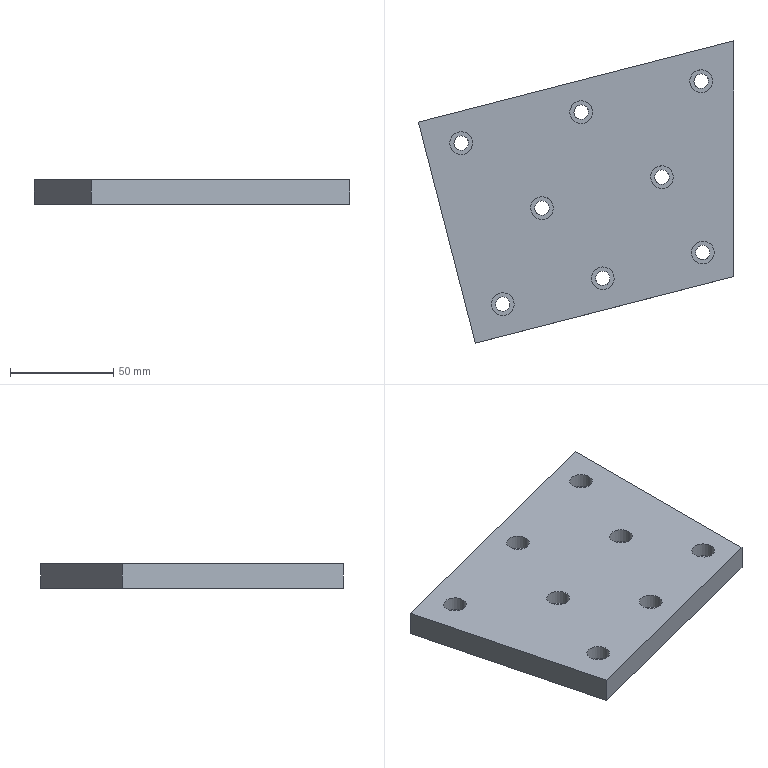Part | STEP file | 车灯-后视镜_id642_x_t | 1 solid | 30 faces | box 152.531 x 146.332 x 12 mm | volume 183119 mm3 | cylinder 16 | plane 14 | commonest cylinder face diameters 7 x8 11 x8
STEP:
#1=CARTESIAN_POINT('',(-249.939,-49.782,-35.286));
#2=VERTEX_POINT('',#1);
#3=CARTESIAN_POINT('',(-249.939,-49.782,-47.286));
#4=VERTEX_POINT('',#3);
#5=CARTESIAN_POINT('',(-249.939,-49.782,-35.286));
#6=DIRECTION('',(0.,0.,-1.));
#7=VECTOR('',#6,1.);
#8=LINE('',#5,#7);
#9=EDGE_CURVE('',#2,#4,#8,.T.);
#10=ORIENTED_EDGE('',*,*,#9,.F.);
#11=CARTESIAN_POINT('',(-277.531,57.217,-35.286));
#12=VERTEX_POINT('',#11);
#13=CARTESIAN_POINT('',(-263.677,3.492,-35.286));
#14=DIRECTION('',(-0.2497,0.9683,0.));
#15=VECTOR('',#14,1.);
#16=LINE('',#13,#15);
#17=EDGE_CURVE('',#2,#12,#16,.T.);
#18=ORIENTED_EDGE('',*,*,#17,.T.);
#19=CARTESIAN_POINT('',(-277.531,57.217,-47.286));
#20=VERTEX_POINT('',#19);
#21=CARTESIAN_POINT('',(-277.531,57.217,-35.286));
#22=DIRECTION('',(0.,0.,-1.));
#23=VECTOR('',#22,1.);
#24=LINE('',#21,#23);
#25=EDGE_CURVE('',#12,#20,#24,.T.);
#26=ORIENTED_EDGE('',*,*,#25,.T.);
#27=CARTESIAN_POINT('',(-263.677,3.492,-47.286));
#28=DIRECTION('',(-0.2497,0.9683,0.));
#29=VECTOR('',#28,1.);
#30=LINE('',#27,#29);
#31=EDGE_CURVE('',#4,#20,#30,.T.);
#32=ORIENTED_EDGE('',*,*,#31,.F.);
#33=EDGE_LOOP('',(#10,#18,#26,#32));
#34=FACE_OUTER_BOUND('',#33,.T.);
#35=CARTESIAN_POINT('',(-249.939,-49.782,-47.286));
#36=DIRECTION('',(-0.9683,-0.2497,0.));
#37=DIRECTION('',(0.2497,-0.9683,0.));
#38=AXIS2_PLACEMENT_3D('',#35,#36,#37);
#39=PLANE('',#38);
#40=ADVANCED_FACE('',(#34),#39,.T.);
#41=CARTESIAN_POINT('',(-125.,96.55,-47.286));
#42=VERTEX_POINT('',#41);
#43=CARTESIAN_POINT('',(-125.,-17.565,-47.286));
#44=VERTEX_POINT('',#43);
#45=CARTESIAN_POINT('',(-125.,0.,-47.286));
#46=DIRECTION('',(0.,-1.,0.));
#47=VECTOR('',#46,1.);
#48=LINE('',#45,#47);
#49=EDGE_CURVE('',#42,#44,#48,.T.);
#50=ORIENTED_EDGE('',*,*,#49,.F.);
#51=CARTESIAN_POINT('',(-125.,96.55,-35.286));
#52=VERTEX_POINT('',#51);
#53=CARTESIAN_POINT('',(-125.,96.55,-35.286));
#54=DIRECTION('',(0.,0.,-1.));
#55=VECTOR('',#54,1.);
#56=LINE('',#53,#55);
#57=EDGE_CURVE('',#52,#42,#56,.T.);
#58=ORIENTED_EDGE('',*,*,#57,.F.);
#59=CARTESIAN_POINT('',(-125.,-17.565,-35.286));
#60=VERTEX_POINT('',#59);
#61=CARTESIAN_POINT('',(-125.,0.,-35.286));
#62=DIRECTION('',(0.,-1.,0.));
#63=VECTOR('',#62,1.);
#64=LINE('',#61,#63);
#65=EDGE_CURVE('',#52,#60,#64,.T.);
#66=ORIENTED_EDGE('',*,*,#65,.T.);
#67=CARTESIAN_POINT('',(-125.,-17.565,-35.286));
#68=DIRECTION('',(0.,0.,-1.));
#69=VECTOR('',#68,1.);
#70=LINE('',#67,#69);
#71=EDGE_CURVE('',#60,#44,#70,.T.);
#72=ORIENTED_EDGE('',*,*,#71,.T.);
#73=EDGE_LOOP('',(#50,#58,#66,#72));
#74=FACE_OUTER_BOUND('',#73,.T.);
#75=CARTESIAN_POINT('',(-125.,0.,-35.286));
#76=DIRECTION('',(1.,0.,0.));
#77=DIRECTION('',(0.,0.,-1.));
#78=AXIS2_PLACEMENT_3D('',#75,#76,#77);
#79=PLANE('',#78);
#80=ADVANCED_FACE('',(#74),#79,.T.);
#81=ORIENTED_EDGE('',*,*,#25,.F.);
#82=CARTESIAN_POINT('',(-109.042,100.665,-35.286));
#83=DIRECTION('',(-0.9683,-0.2497,0.));
#84=VECTOR('',#83,1.);
#85=LINE('',#82,#84);
#86=EDGE_CURVE('',#52,#12,#85,.T.);
#87=ORIENTED_EDGE('',*,*,#86,.F.);
#88=ORIENTED_EDGE('',*,*,#57,.T.);
#89=CARTESIAN_POINT('',(-109.042,100.665,-47.286));
#90=DIRECTION('',(-0.9683,-0.2497,0.));
#91=VECTOR('',#90,1.);
#92=LINE('',#89,#91);
#93=EDGE_CURVE('',#42,#20,#92,.T.);
#94=ORIENTED_EDGE('',*,*,#93,.T.);
#95=EDGE_LOOP('',(#81,#87,#88,#94));
#96=FACE_OUTER_BOUND('',#95,.T.);
#97=CARTESIAN_POINT('',(-109.042,100.665,-35.286));
#98=DIRECTION('',(0.2497,-0.9683,0.));
#99=DIRECTION('',(0.9683,0.2497,0.));
#100=AXIS2_PLACEMENT_3D('',#97,#98,#99);
#101=PLANE('',#100);
#102=ADVANCED_FACE('',(#96),#101,.F.);
#103=CARTESIAN_POINT('',(-81.451,-6.335,-35.286));
#104=DIRECTION('',(-0.9683,-0.2497,0.));
#105=VECTOR('',#104,1.);
#106=LINE('',#103,#105);
#107=EDGE_CURVE('',#60,#2,#106,.T.);
#108=ORIENTED_EDGE('',*,*,#107,.T.);
#109=ORIENTED_EDGE('',*,*,#9,.T.);
#110=CARTESIAN_POINT('',(-81.451,-6.335,-47.286));
#111=DIRECTION('',(-0.9683,-0.2497,0.));
#112=VECTOR('',#111,1.);
#113=LINE('',#110,#112);
#114=EDGE_CURVE('',#44,#4,#113,.T.);
#115=ORIENTED_EDGE('',*,*,#114,.F.);
#116=ORIENTED_EDGE('',*,*,#71,.F.);
#117=EDGE_LOOP('',(#108,#109,#115,#116));
#118=FACE_OUTER_BOUND('',#117,.T.);
#119=CARTESIAN_POINT('',(-81.451,-6.335,-35.286));
#120=DIRECTION('',(0.2497,-0.9683,0.));
#121=DIRECTION('',(0.9683,0.2497,0.));
#122=AXIS2_PLACEMENT_3D('',#119,#120,#121);
#123=PLANE('',#122);
#124=ADVANCED_FACE('',(#118),#123,.T.);
#125=CARTESIAN_POINT('',(-197.367,56.718,-35.286));
#126=VERTEX_POINT('',#125);
#127=CARTESIAN_POINT('',(-198.74,62.044,-35.286));
#128=DIRECTION('',(0.,0.,-1.));
#129=DIRECTION('',(0.2497,-0.9683,0.));
#130=AXIS2_PLACEMENT_3D('',#127,#128,#129);
#131=CIRCLE('',#130,5.5);
#132=EDGE_CURVE('',#126,#126,#131,.T.);
#133=ORIENTED_EDGE('',*,*,#132,.T.);
#134=EDGE_LOOP('',(#133));
#135=FACE_BOUND('',#134,.T.);
#136=CARTESIAN_POINT('',(-138.533,-11.244,-35.286));
#137=VERTEX_POINT('',#136);
#138=CARTESIAN_POINT('',(-139.906,-5.918,-35.286));
#139=DIRECTION('',(0.,0.,-1.));
#140=DIRECTION('',(0.2497,-0.9683,0.));
#141=AXIS2_PLACEMENT_3D('',#138,#139,#140);
#142=CIRCLE('',#141,5.5);
#143=EDGE_CURVE('',#137,#137,#142,.T.);
#144=ORIENTED_EDGE('',*,*,#143,.T.);
#145=EDGE_LOOP('',(#144));
#146=FACE_BOUND('',#145,.T.);
#147=CARTESIAN_POINT('',(-186.949,-23.729,-35.286));
#148=VERTEX_POINT('',#147);
#149=CARTESIAN_POINT('',(-188.322,-18.403,-35.286));
#150=DIRECTION('',(0.,0.,-1.));
#151=DIRECTION('',(0.2497,-0.9683,0.));
#152=AXIS2_PLACEMENT_3D('',#149,#150,#151);
#153=CIRCLE('',#152,5.5);
#154=EDGE_CURVE('',#148,#148,#153,.T.);
#155=ORIENTED_EDGE('',*,*,#154,.T.);
#156=EDGE_LOOP('',(#155));
#157=FACE_BOUND('',#156,.T.);
#158=CARTESIAN_POINT('',(-158.267,25.234,-35.286));
#159=VERTEX_POINT('',#158);
#160=CARTESIAN_POINT('',(-159.64,30.56,-35.286));
#161=DIRECTION('',(0.,0.,-1.));
#162=DIRECTION('',(0.2497,-0.9683,0.));
#163=AXIS2_PLACEMENT_3D('',#160,#161,#162);
#164=CIRCLE('',#163,5.5);
#165=EDGE_CURVE('',#159,#159,#164,.T.);
#166=ORIENTED_EDGE('',*,*,#165,.T.);
#167=EDGE_LOOP('',(#166));
#168=FACE_BOUND('',#167,.T.);
#169=CARTESIAN_POINT('',(-216.366,10.252,-35.286));
#170=VERTEX_POINT('',#169);
#171=CARTESIAN_POINT('',(-217.739,15.578,-35.286));
#172=DIRECTION('',(0.,0.,-1.));
#173=DIRECTION('',(0.2497,-0.9683,0.));
#174=AXIS2_PLACEMENT_3D('',#171,#172,#173);
#175=CIRCLE('',#174,5.5);
#176=EDGE_CURVE('',#170,#170,#175,.T.);
#177=ORIENTED_EDGE('',*,*,#176,.T.);
#178=EDGE_LOOP('',(#177));
#179=FACE_BOUND('',#178,.T.);
#180=CARTESIAN_POINT('',(-235.365,-36.214,-35.286));
#181=VERTEX_POINT('',#180);
#182=CARTESIAN_POINT('',(-236.739,-30.888,-35.286));
#183=DIRECTION('',(0.,0.,-1.));
#184=DIRECTION('',(0.2497,-0.9683,0.));
#185=AXIS2_PLACEMENT_3D('',#182,#183,#184);
#186=CIRCLE('',#185,5.5);
#187=EDGE_CURVE('',#181,#181,#186,.T.);
#188=ORIENTED_EDGE('',*,*,#187,.T.);
#189=EDGE_LOOP('',(#188));
#190=FACE_BOUND('',#189,.T.);
#191=CARTESIAN_POINT('',(-255.466,41.736,-35.286));
#192=VERTEX_POINT('',#191);
#193=CARTESIAN_POINT('',(-256.839,47.062,-35.286));
#194=DIRECTION('',(0.,0.,-1.));
#195=DIRECTION('',(0.2497,-0.9683,0.));
#196=AXIS2_PLACEMENT_3D('',#193,#194,#195);
#197=CIRCLE('',#196,5.5);
#198=EDGE_CURVE('',#192,#192,#197,.T.);
#199=ORIENTED_EDGE('',*,*,#198,.T.);
#200=EDGE_LOOP('',(#199));
#201=FACE_BOUND('',#200,.T.);
#202=CARTESIAN_POINT('',(-139.267,71.7,-35.286));
#203=VERTEX_POINT('',#202);
#204=CARTESIAN_POINT('',(-140.641,77.026,-35.286));
#205=DIRECTION('',(0.,0.,-1.));
#206=DIRECTION('',(0.2497,-0.9683,0.));
#207=AXIS2_PLACEMENT_3D('',#204,#205,#206);
#208=CIRCLE('',#207,5.5);
#209=EDGE_CURVE('',#203,#203,#208,.T.);
#210=ORIENTED_EDGE('',*,*,#209,.T.);
#211=EDGE_LOOP('',(#210));
#212=FACE_BOUND('',#211,.T.);
#213=ORIENTED_EDGE('',*,*,#17,.F.);
#214=ORIENTED_EDGE('',*,*,#107,.F.);
#215=ORIENTED_EDGE('',*,*,#65,.F.);
#216=ORIENTED_EDGE('',*,*,#86,.T.);
#217=EDGE_LOOP('',(#213,#214,#215,#216));
#218=FACE_BOUND('',#217,.T.);
#219=CARTESIAN_POINT('',(-95.188,46.94,-35.286));
#220=DIRECTION('',(0.,0.,-1.));
#221=DIRECTION('',(0.9683,0.2497,0.));
#222=AXIS2_PLACEMENT_3D('',#219,#220,#221);
#223=PLANE('',#222);
#224=ADVANCED_FACE('',(#135,#146,#157,#168,#179,#190,#201,#212,#218),#223,.F.);
#225=CARTESIAN_POINT('',(-199.614,65.433,-47.286));
#226=VERTEX_POINT('',#225);
#227=CARTESIAN_POINT('',(-198.74,62.044,-47.286));
#228=DIRECTION('',(0.,0.,1.));
#229=DIRECTION('',(-0.2497,0.9683,0.));
#230=AXIS2_PLACEMENT_3D('',#227,#228,#229);
#231=CIRCLE('',#230,3.5);
#232=EDGE_CURVE('',#226,#226,#231,.T.);
#233=ORIENTED_EDGE('',*,*,#232,.T.);
#234=EDGE_LOOP('',(#233));
#235=FACE_BOUND('',#234,.T.);
#236=CARTESIAN_POINT('',(-140.78,-2.529,-47.286));
#237=VERTEX_POINT('',#236);
#238=CARTESIAN_POINT('',(-139.906,-5.918,-47.286));
#239=DIRECTION('',(0.,0.,1.));
#240=DIRECTION('',(-0.2497,0.9683,0.));
#241=AXIS2_PLACEMENT_3D('',#238,#239,#240);
#242=CIRCLE('',#241,3.5);
#243=EDGE_CURVE('',#237,#237,#242,.T.);
#244=ORIENTED_EDGE('',*,*,#243,.T.);
#245=EDGE_LOOP('',(#244));
#246=FACE_BOUND('',#245,.T.);
#247=CARTESIAN_POINT('',(-189.196,-15.014,-47.286));
#248=VERTEX_POINT('',#247);
#249=CARTESIAN_POINT('',(-188.322,-18.403,-47.286));
#250=DIRECTION('',(0.,0.,1.));
#251=DIRECTION('',(-0.2497,0.9683,0.));
#252=AXIS2_PLACEMENT_3D('',#249,#250,#251);
#253=CIRCLE('',#252,3.5);
#254=EDGE_CURVE('',#248,#248,#253,.T.);
#255=ORIENTED_EDGE('',*,*,#254,.T.);
#256=EDGE_LOOP('',(#255));
#257=FACE_BOUND('',#256,.T.);
#258=CARTESIAN_POINT('',(-160.514,33.949,-47.286));
#259=VERTEX_POINT('',#258);
#260=CARTESIAN_POINT('',(-159.64,30.56,-47.286));
#261=DIRECTION('',(0.,0.,1.));
#262=DIRECTION('',(-0.2497,0.9683,0.));
#263=AXIS2_PLACEMENT_3D('',#260,#261,#262);
#264=CIRCLE('',#263,3.5);
#265=EDGE_CURVE('',#259,#259,#264,.T.);
#266=ORIENTED_EDGE('',*,*,#265,.T.);
#267=EDGE_LOOP('',(#266));
#268=FACE_BOUND('',#267,.T.);
#269=CARTESIAN_POINT('',(-218.613,18.967,-47.286));
#270=VERTEX_POINT('',#269);
#271=CARTESIAN_POINT('',(-217.739,15.578,-47.286));
#272=DIRECTION('',(0.,0.,1.));
#273=DIRECTION('',(-0.2497,0.9683,0.));
#274=AXIS2_PLACEMENT_3D('',#271,#272,#273);
#275=CIRCLE('',#274,3.5);
#276=EDGE_CURVE('',#270,#270,#275,.T.);
#277=ORIENTED_EDGE('',*,*,#276,.T.);
#278=EDGE_LOOP('',(#277));
#279=FACE_BOUND('',#278,.T.);
#280=CARTESIAN_POINT('',(-237.613,-27.499,-47.286));
#281=VERTEX_POINT('',#280);
#282=CARTESIAN_POINT('',(-236.739,-30.888,-47.286));
#283=DIRECTION('',(0.,0.,1.));
#284=DIRECTION('',(-0.2497,0.9683,0.));
#285=AXIS2_PLACEMENT_3D('',#282,#283,#284);
#286=CIRCLE('',#285,3.5);
#287=EDGE_CURVE('',#281,#281,#286,.T.);
#288=ORIENTED_EDGE('',*,*,#287,.T.);
#289=EDGE_LOOP('',(#288));
#290=FACE_BOUND('',#289,.T.);
#291=CARTESIAN_POINT('',(-257.713,50.451,-47.286));
#292=VERTEX_POINT('',#291);
#293=CARTESIAN_POINT('',(-256.839,47.062,-47.286));
#294=DIRECTION('',(0.,0.,1.));
#295=DIRECTION('',(-0.2497,0.9683,0.));
#296=AXIS2_PLACEMENT_3D('',#293,#294,#295);
#297=CIRCLE('',#296,3.5);
#298=EDGE_CURVE('',#292,#292,#297,.T.);
#299=ORIENTED_EDGE('',*,*,#298,.T.);
#300=EDGE_LOOP('',(#299));
#301=FACE_BOUND('',#300,.T.);
#302=CARTESIAN_POINT('',(-141.515,80.415,-47.286));
#303=VERTEX_POINT('',#302);
#304=CARTESIAN_POINT('',(-140.641,77.026,-47.286));
#305=DIRECTION('',(0.,0.,1.));
#306=DIRECTION('',(-0.2497,0.9683,0.));
#307=AXIS2_PLACEMENT_3D('',#304,#305,#306);
#308=CIRCLE('',#307,3.5);
#309=EDGE_CURVE('',#303,#303,#308,.T.);
#310=ORIENTED_EDGE('',*,*,#309,.T.);
#311=EDGE_LOOP('',(#310));
#312=FACE_BOUND('',#311,.T.);
#313=ORIENTED_EDGE('',*,*,#114,.T.);
#314=ORIENTED_EDGE('',*,*,#31,.T.);
#315=ORIENTED_EDGE('',*,*,#93,.F.);
#316=ORIENTED_EDGE('',*,*,#49,.T.);
#317=EDGE_LOOP('',(#313,#314,#315,#316));
#318=FACE_BOUND('',#317,.T.);
#319=CARTESIAN_POINT('',(-95.188,46.94,-47.286));
#320=DIRECTION('',(0.,0.,-1.));
#321=DIRECTION('',(0.9683,0.2497,0.));
#322=AXIS2_PLACEMENT_3D('',#319,#320,#321);
#323=PLANE('',#322);
#324=ADVANCED_FACE('',(#235,#246,#257,#268,#279,#290,#301,#312,#318),#323,.T.);
#325=CARTESIAN_POINT('',(-144.141,77.026,-42.286));
#326=VERTEX_POINT('',#325);
#327=CARTESIAN_POINT('',(-140.641,77.026,-42.286));
#328=DIRECTION('',(0.,0.,1.));
#329=DIRECTION('',(-1.,0.,0.));
#330=AXIS2_PLACEMENT_3D('',#327,#328,#329);
#331=CIRCLE('',#330,3.5);
#332=EDGE_CURVE('',#326,#326,#331,.T.);
#333=ORIENTED_EDGE('',*,*,#332,.T.);
#334=EDGE_LOOP('',(#333));
#335=FACE_BOUND('',#334,.T.);
#336=ORIENTED_EDGE('',*,*,#309,.F.);
#337=EDGE_LOOP('',(#336));
#338=FACE_BOUND('',#337,.T.);
#339=CARTESIAN_POINT('',(-140.641,77.026,-47.286));
#340=DIRECTION('',(0.,0.,1.));
#341=DIRECTION('',(-0.2497,0.9683,0.));
#342=AXIS2_PLACEMENT_3D('',#339,#340,#341);
#343=CYLINDRICAL_SURFACE('',#342,3.5);
#344=ADVANCED_FACE('',(#335,#338),#343,.F.);
#345=ORIENTED_EDGE('',*,*,#332,.F.);
#346=EDGE_LOOP('',(#345));
#347=FACE_BOUND('',#346,.T.);
#348=CARTESIAN_POINT('',(-142.014,82.352,-42.286));
#349=VERTEX_POINT('',#348);
#350=CARTESIAN_POINT('',(-140.641,77.026,-42.286));
#351=DIRECTION('',(0.,0.,1.));
#352=DIRECTION('',(-0.2497,0.9683,0.));
#353=AXIS2_PLACEMENT_3D('',#350,#351,#352);
#354=CIRCLE('',#353,5.5);
#355=EDGE_CURVE('',#349,#349,#354,.T.);
#356=ORIENTED_EDGE('',*,*,#355,.T.);
#357=EDGE_LOOP('',(#356));
#358=FACE_BOUND('',#357,.T.);
#359=CARTESIAN_POINT('',(-140.641,77.026,-42.286));
#360=DIRECTION('',(0.,0.,-1.));
#361=DIRECTION('',(0.2497,-0.9683,0.));
#362=AXIS2_PLACEMENT_3D('',#359,#360,#361);
#363=PLANE('',#362);
#364=ADVANCED_FACE('',(#347,#358),#363,.F.);
#365=ORIENTED_EDGE('',*,*,#355,.F.);
#366=EDGE_LOOP('',(#365));
#367=FACE_BOUND('',#366,.T.);
#368=ORIENTED_EDGE('',*,*,#209,.F.);
#369=EDGE_LOOP('',(#368));
#370=FACE_BOUND('',#369,.T.);
#371=CARTESIAN_POINT('',(-140.641,77.026,-35.286));
#372=DIRECTION('',(0.,0.,-1.));
#373=DIRECTION('',(0.2497,-0.9683,0.));
#374=AXIS2_PLACEMENT_3D('',#371,#372,#373);
#375=CYLINDRICAL_SURFACE('',#374,5.5);
#376=ADVANCED_FACE('',(#367,#370),#375,.F.);
#377=CARTESIAN_POINT('',(-260.339,47.062,-42.286));
#378=VERTEX_POINT('',#377);
#379=CARTESIAN_POINT('',(-256.839,47.062,-42.286));
#380=DIRECTION('',(0.,0.,1.));
#381=DIRECTION('',(-1.,0.,0.));
#382=AXIS2_PLACEMENT_3D('',#379,#380,#381);
#383=CIRCLE('',#382,3.5);
#384=EDGE_CURVE('',#378,#378,#383,.T.);
#385=ORIENTED_EDGE('',*,*,#384,.T.);
#386=EDGE_LOOP('',(#385));
#387=FACE_BOUND('',#386,.T.);
#388=ORIENTED_EDGE('',*,*,#298,.F.);
#389=EDGE_LOOP('',(#388));
#390=FACE_BOUND('',#389,.T.);
#391=CARTESIAN_POINT('',(-256.839,47.062,-47.286));
#392=DIRECTION('',(0.,0.,1.));
#393=DIRECTION('',(-0.2497,0.9683,0.));
#394=AXIS2_PLACEMENT_3D('',#391,#392,#393);
#395=CYLINDRICAL_SURFACE('',#394,3.5);
#396=ADVANCED_FACE('',(#387,#390),#395,.F.);
#397=ORIENTED_EDGE('',*,*,#384,.F.);
#398=EDGE_LOOP('',(#397));
#399=FACE_BOUND('',#398,.T.);
#400=CARTESIAN_POINT('',(-258.213,52.388,-42.286));
#401=VERTEX_POINT('',#400);
#402=CARTESIAN_POINT('',(-256.839,47.062,-42.286));
#403=DIRECTION('',(0.,0.,1.));
#404=DIRECTION('',(-0.2497,0.9683,0.));
#405=AXIS2_PLACEMENT_3D('',#402,#403,#404);
#406=CIRCLE('',#405,5.5);
#407=EDGE_CURVE('',#401,#401,#406,.T.);
#408=ORIENTED_EDGE('',*,*,#407,.T.);
#409=EDGE_LOOP('',(#408));
#410=FACE_BOUND('',#409,.T.);
#411=CARTESIAN_POINT('',(-256.839,47.062,-42.286));
#412=DIRECTION('',(0.,0.,-1.));
#413=DIRECTION('',(0.2497,-0.9683,0.));
#414=AXIS2_PLACEMENT_3D('',#411,#412,#413);
#415=PLANE('',#414);
#416=ADVANCED_FACE('',(#399,#410),#415,.F.);
#417=ORIENTED_EDGE('',*,*,#407,.F.);
#418=EDGE_LOOP('',(#417));
#419=FACE_BOUND('',#418,.T.);
#420=ORIENTED_EDGE('',*,*,#198,.F.);
#421=EDGE_LOOP('',(#420));
#422=FACE_BOUND('',#421,.T.);
#423=CARTESIAN_POINT('',(-256.839,47.062,-35.286));
#424=DIRECTION('',(0.,0.,-1.));
#425=DIRECTION('',(0.2497,-0.9683,0.));
#426=AXIS2_PLACEMENT_3D('',#423,#424,#425);
#427=CYLINDRICAL_SURFACE('',#426,5.5);
#428=ADVANCED_FACE('',(#419,#422),#427,.F.);
#429=CARTESIAN_POINT('',(-240.239,-30.888,-42.286));
#430=VERTEX_POINT('',#429);
#431=CARTESIAN_POINT('',(-236.739,-30.888,-42.286));
#432=DIRECTION('',(0.,0.,1.));
#433=DIRECTION('',(-1.,0.,0.));
#434=AXIS2_PLACEMENT_3D('',#431,#432,#433);
#435=CIRCLE('',#434,3.5);
#436=EDGE_CURVE('',#430,#430,#435,.T.);
#437=ORIENTED_EDGE('',*,*,#436,.T.);
#438=EDGE_LOOP('',(#437));
#439=FACE_BOUND('',#438,.T.);
#440=ORIENTED_EDGE('',*,*,#287,.F.);
#441=EDGE_LOOP('',(#440));
#442=FACE_BOUND('',#441,.T.);
#443=CARTESIAN_POINT('',(-236.739,-30.888,-47.286));
#444=DIRECTION('',(0.,0.,1.));
#445=DIRECTION('',(-0.2497,0.9683,0.));
#446=AXIS2_PLACEMENT_3D('',#443,#444,#445);
#447=CYLINDRICAL_SURFACE('',#446,3.5);
#448=ADVANCED_FACE('',(#439,#442),#447,.F.);
#449=ORIENTED_EDGE('',*,*,#436,.F.);
#450=EDGE_LOOP('',(#449));
#451=FACE_BOUND('',#450,.T.);
#452=CARTESIAN_POINT('',(-238.112,-25.562,-42.286));
#453=VERTEX_POINT('',#452);
#454=CARTESIAN_POINT('',(-236.739,-30.888,-42.286));
#455=DIRECTION('',(0.,0.,1.));
#456=DIRECTION('',(-0.2497,0.9683,0.));
#457=AXIS2_PLACEMENT_3D('',#454,#455,#456);
#458=CIRCLE('',#457,5.5);
#459=EDGE_CURVE('',#453,#453,#458,.T.);
#460=ORIENTED_EDGE('',*,*,#459,.T.);
#461=EDGE_LOOP('',(#460));
#462=FACE_BOUND('',#461,.T.);
#463=CARTESIAN_POINT('',(-236.739,-30.888,-42.286));
#464=DIRECTION('',(0.,0.,-1.));
#465=DIRECTION('',(0.2497,-0.9683,0.));
#466=AXIS2_PLACEMENT_3D('',#463,#464,#465);
#467=PLANE('',#466);
#468=ADVANCED_FACE('',(#451,#462),#467,.F.);
#469=ORIENTED_EDGE('',*,*,#459,.F.);
#470=EDGE_LOOP('',(#469));
#471=FACE_BOUND('',#470,.T.);
#472=ORIENTED_EDGE('',*,*,#187,.F.);
#473=EDGE_LOOP('',(#472));
#474=FACE_BOUND('',#473,.T.);
#475=CARTESIAN_POINT('',(-236.739,-30.888,-35.286));
#476=DIRECTION('',(0.,0.,-1.));
#477=DIRECTION('',(0.2497,-0.9683,0.));
#478=AXIS2_PLACEMENT_3D('',#475,#476,#477);
#479=CYLINDRICAL_SURFACE('',#478,5.5);
#480=ADVANCED_FACE('',(#471,#474),#479,.F.);
#481=CARTESIAN_POINT('',(-221.239,15.578,-42.286));
#482=VERTEX_POINT('',#481);
#483=CARTESIAN_POINT('',(-217.739,15.578,-42.286));
#484=DIRECTION('',(0.,0.,1.));
#485=DIRECTION('',(-1.,0.,0.));
#486=AXIS2_PLACEMENT_3D('',#483,#484,#485);
#487=CIRCLE('',#486,3.5);
#488=EDGE_CURVE('',#482,#482,#487,.T.);
#489=ORIENTED_EDGE('',*,*,#488,.T.);
#490=EDGE_LOOP('',(#489));
#491=FACE_BOUND('',#490,.T.);
#492=ORIENTED_EDGE('',*,*,#276,.F.);
#493=EDGE_LOOP('',(#492));
#494=FACE_BOUND('',#493,.T.);
#495=CARTESIAN_POINT('',(-217.739,15.578,-47.286));
#496=DIRECTION('',(0.,0.,1.));
#497=DIRECTION('',(-0.2497,0.9683,0.));
#498=AXIS2_PLACEMENT_3D('',#495,#496,#497);
#499=CYLINDRICAL_SURFACE('',#498,3.5);
#500=ADVANCED_FACE('',(#491,#494),#499,.F.);
#501=ORIENTED_EDGE('',*,*,#488,.F.);
#502=EDGE_LOOP('',(#501));
#503=FACE_BOUND('',#502,.T.);
#504=CARTESIAN_POINT('',(-219.113,20.904,-42.286));
#505=VERTEX_POINT('',#504);
#506=CARTESIAN_POINT('',(-217.739,15.578,-42.286));
#507=DIRECTION('',(0.,0.,1.));
#508=DIRECTION('',(-0.2497,0.9683,0.));
#509=AXIS2_PLACEMENT_3D('',#506,#507,#508);
#510=CIRCLE('',#509,5.5);
#511=EDGE_CURVE('',#505,#505,#510,.T.);
#512=ORIENTED_EDGE('',*,*,#511,.T.);
#513=EDGE_LOOP('',(#512));
#514=FACE_BOUND('',#513,.T.);
#515=CARTESIAN_POINT('',(-217.739,15.578,-42.286));
#516=DIRECTION('',(0.,0.,-1.));
#517=DIRECTION('',(0.2497,-0.9683,0.));
#518=AXIS2_PLACEMENT_3D('',#515,#516,#517);
#519=PLANE('',#518);
#520=ADVANCED_FACE('',(#503,#514),#519,.F.);
#521=ORIENTED_EDGE('',*,*,#511,.F.);
#522=EDGE_LOOP('',(#521));
#523=FACE_BOUND('',#522,.T.);
#524=ORIENTED_EDGE('',*,*,#176,.F.);
#525=EDGE_LOOP('',(#524));
#526=FACE_BOUND('',#525,.T.);
#527=CARTESIAN_POINT('',(-217.739,15.578,-35.286));
#528=DIRECTION('',(0.,0.,-1.));
#529=DIRECTION('',(0.2497,-0.9683,0.));
#530=AXIS2_PLACEMENT_3D('',#527,#528,#529);
#531=CYLINDRICAL_SURFACE('',#530,5.5);
#532=ADVANCED_FACE('',(#523,#526),#531,.F.);
#533=CARTESIAN_POINT('',(-163.14,30.56,-42.286));
#534=VERTEX_POINT('',#533);
#535=CARTESIAN_POINT('',(-159.64,30.56,-42.286));
#536=DIRECTION('',(0.,0.,1.));
#537=DIRECTION('',(-1.,0.,0.));
#538=AXIS2_PLACEMENT_3D('',#535,#536,#537);
#539=CIRCLE('',#538,3.5);
#540=EDGE_CURVE('',#534,#534,#539,.T.);
#541=ORIENTED_EDGE('',*,*,#540,.T.);
#542=EDGE_LOOP('',(#541));
#543=FACE_BOUND('',#542,.T.);
#544=ORIENTED_EDGE('',*,*,#265,.F.);
#545=EDGE_LOOP('',(#544));
#546=FACE_BOUND('',#545,.T.);
#547=CARTESIAN_POINT('',(-159.64,30.56,-47.286));
#548=DIRECTION('',(0.,0.,1.));
#549=DIRECTION('',(-0.2497,0.9683,0.));
#550=AXIS2_PLACEMENT_3D('',#547,#548,#549);
#551=CYLINDRICAL_SURFACE('',#550,3.5);
#552=ADVANCED_FACE('',(#543,#546),#551,.F.);
#553=ORIENTED_EDGE('',*,*,#540,.F.);
#554=EDGE_LOOP('',(#553));
#555=FACE_BOUND('',#554,.T.);
#556=CARTESIAN_POINT('',(-161.013,35.886,-42.286));
#557=VERTEX_POINT('',#556);
#558=CARTESIAN_POINT('',(-159.64,30.56,-42.286));
#559=DIRECTION('',(0.,0.,1.));
#560=DIRECTION('',(-0.2497,0.9683,0.));
#561=AXIS2_PLACEMENT_3D('',#558,#559,#560);
#562=CIRCLE('',#561,5.5);
#563=EDGE_CURVE('',#557,#557,#562,.T.);
#564=ORIENTED_EDGE('',*,*,#563,.T.);
#565=EDGE_LOOP('',(#564));
#566=FACE_BOUND('',#565,.T.);
#567=CARTESIAN_POINT('',(-159.64,30.56,-42.286));
#568=DIRECTION('',(0.,0.,-1.));
#569=DIRECTION('',(0.2497,-0.9683,0.));
#570=AXIS2_PLACEMENT_3D('',#567,#568,#569);
#571=PLANE('',#570);
#572=ADVANCED_FACE('',(#555,#566),#571,.F.);
#573=ORIENTED_EDGE('',*,*,#563,.F.);
#574=EDGE_LOOP('',(#573));
#575=FACE_BOUND('',#574,.T.);
#576=ORIENTED_EDGE('',*,*,#165,.F.);
#577=EDGE_LOOP('',(#576));
#578=FACE_BOUND('',#577,.T.);
#579=CARTESIAN_POINT('',(-159.64,30.56,-35.286));
#580=DIRECTION('',(0.,0.,-1.));
#581=DIRECTION('',(0.2497,-0.9683,0.));
#582=AXIS2_PLACEMENT_3D('',#579,#580,#581);
#583=CYLINDRICAL_SURFACE('',#582,5.5);
#584=ADVANCED_FACE('',(#575,#578),#583,.F.);
#585=CARTESIAN_POINT('',(-191.822,-18.403,-42.286));
#586=VERTEX_POINT('',#585);
#587=CARTESIAN_POINT('',(-188.322,-18.403,-42.286));
#588=DIRECTION('',(0.,0.,1.));
#589=DIRECTION('',(-1.,0.,0.));
#590=AXIS2_PLACEMENT_3D('',#587,#588,#589);
#591=CIRCLE('',#590,3.5);
#592=EDGE_CURVE('',#586,#586,#591,.T.);
#593=ORIENTED_EDGE('',*,*,#592,.T.);
#594=EDGE_LOOP('',(#593));
#595=FACE_BOUND('',#594,.T.);
#596=ORIENTED_EDGE('',*,*,#254,.F.);
#597=EDGE_LOOP('',(#596));
#598=FACE_BOUND('',#597,.T.);
#599=CARTESIAN_POINT('',(-188.322,-18.403,-47.286));
#600=DIRECTION('',(0.,0.,1.));
#601=DIRECTION('',(-0.2497,0.9683,0.));
#602=AXIS2_PLACEMENT_3D('',#599,#600,#601);
#603=CYLINDRICAL_SURFACE('',#602,3.5);
#604=ADVANCED_FACE('',(#595,#598),#603,.F.);
#605=ORIENTED_EDGE('',*,*,#592,.F.);
#606=EDGE_LOOP('',(#605));
#607=FACE_BOUND('',#606,.T.);
#608=CARTESIAN_POINT('',(-189.696,-13.077,-42.286));
#609=VERTEX_POINT('',#608);
#610=CARTESIAN_POINT('',(-188.322,-18.403,-42.286));
#611=DIRECTION('',(0.,0.,1.));
#612=DIRECTION('',(-0.2497,0.9683,0.));
#613=AXIS2_PLACEMENT_3D('',#610,#611,#612);
#614=CIRCLE('',#613,5.5);
#615=EDGE_CURVE('',#609,#609,#614,.T.);
#616=ORIENTED_EDGE('',*,*,#615,.T.);
#617=EDGE_LOOP('',(#616));
#618=FACE_BOUND('',#617,.T.);
#619=CARTESIAN_POINT('',(-188.322,-18.403,-42.286));
#620=DIRECTION('',(0.,0.,-1.));
#621=DIRECTION('',(0.2497,-0.9683,0.));
#622=AXIS2_PLACEMENT_3D('',#619,#620,#621);
#623=PLANE('',#622);
#624=ADVANCED_FACE('',(#607,#618),#623,.F.);
#625=ORIENTED_EDGE('',*,*,#615,.F.);
#626=EDGE_LOOP('',(#625));
#627=FACE_BOUND('',#626,.T.);
#628=ORIENTED_EDGE('',*,*,#154,.F.);
#629=EDGE_LOOP('',(#628));
#630=FACE_BOUND('',#629,.T.);
#631=CARTESIAN_POINT('',(-188.322,-18.403,-35.286));
#632=DIRECTION('',(0.,0.,-1.));
#633=DIRECTION('',(0.2497,-0.9683,0.));
#634=AXIS2_PLACEMENT_3D('',#631,#632,#633);
#635=CYLINDRICAL_SURFACE('',#634,5.5);
#636=ADVANCED_FACE('',(#627,#630),#635,.F.);
#637=CARTESIAN_POINT('',(-143.406,-5.918,-42.286));
#638=VERTEX_POINT('',#637);
#639=CARTESIAN_POINT('',(-139.906,-5.918,-42.286));
#640=DIRECTION('',(0.,0.,1.));
#641=DIRECTION('',(-1.,0.,0.));
#642=AXIS2_PLACEMENT_3D('',#639,#640,#641);
#643=CIRCLE('',#642,3.5);
#644=EDGE_CURVE('',#638,#638,#643,.T.);
#645=ORIENTED_EDGE('',*,*,#644,.T.);
#646=EDGE_LOOP('',(#645));
#647=FACE_BOUND('',#646,.T.);
#648=ORIENTED_EDGE('',*,*,#243,.F.);
#649=EDGE_LOOP('',(#648));
#650=FACE_BOUND('',#649,.T.);
#651=CARTESIAN_POINT('',(-139.906,-5.918,-47.286));
#652=DIRECTION('',(0.,0.,1.));
#653=DIRECTION('',(-0.2497,0.9683,0.));
#654=AXIS2_PLACEMENT_3D('',#651,#652,#653);
#655=CYLINDRICAL_SURFACE('',#654,3.5);
#656=ADVANCED_FACE('',(#647,#650),#655,.F.);
#657=ORIENTED_EDGE('',*,*,#644,.F.);
#658=EDGE_LOOP('',(#657));
#659=FACE_BOUND('',#658,.T.);
#660=CARTESIAN_POINT('',(-141.28,-0.5922,-42.286));
#661=VERTEX_POINT('',#660);
#662=CARTESIAN_POINT('',(-139.906,-5.918,-42.286));
#663=DIRECTION('',(0.,0.,1.));
#664=DIRECTION('',(-0.2497,0.9683,0.));
#665=AXIS2_PLACEMENT_3D('',#662,#663,#664);
#666=CIRCLE('',#665,5.5);
#667=EDGE_CURVE('',#661,#661,#666,.T.);
#668=ORIENTED_EDGE('',*,*,#667,.T.);
#669=EDGE_LOOP('',(#668));
#670=FACE_BOUND('',#669,.T.);
#671=CARTESIAN_POINT('',(-139.906,-5.918,-42.286));
#672=DIRECTION('',(0.,0.,-1.));
#673=DIRECTION('',(0.2497,-0.9683,0.));
#674=AXIS2_PLACEMENT_3D('',#671,#672,#673);
#675=PLANE('',#674);
#676=ADVANCED_FACE('',(#659,#670),#675,.F.);
#677=ORIENTED_EDGE('',*,*,#667,.F.);
#678=EDGE_LOOP('',(#677));
#679=FACE_BOUND('',#678,.T.);
#680=ORIENTED_EDGE('',*,*,#143,.F.);
#681=EDGE_LOOP('',(#680));
#682=FACE_BOUND('',#681,.T.);
#683=CARTESIAN_POINT('',(-139.906,-5.918,-35.286));
#684=DIRECTION('',(0.,0.,-1.));
#685=DIRECTION('',(0.2497,-0.9683,0.));
#686=AXIS2_PLACEMENT_3D('',#683,#684,#685);
#687=CYLINDRICAL_SURFACE('',#686,5.5);
#688=ADVANCED_FACE('',(#679,#682),#687,.F.);
#689=CARTESIAN_POINT('',(-202.24,62.044,-42.286));
#690=VERTEX_POINT('',#689);
#691=CARTESIAN_POINT('',(-198.74,62.044,-42.286));
#692=DIRECTION('',(0.,0.,1.));
#693=DIRECTION('',(-1.,0.,0.));
#694=AXIS2_PLACEMENT_3D('',#691,#692,#693);
#695=CIRCLE('',#694,3.5);
#696=EDGE_CURVE('',#690,#690,#695,.T.);
#697=ORIENTED_EDGE('',*,*,#696,.T.);
#698=EDGE_LOOP('',(#697));
#699=FACE_BOUND('',#698,.T.);
#700=ORIENTED_EDGE('',*,*,#232,.F.);
#701=EDGE_LOOP('',(#700));
#702=FACE_BOUND('',#701,.T.);
#703=CARTESIAN_POINT('',(-198.74,62.044,-47.286));
#704=DIRECTION('',(0.,0.,1.));
#705=DIRECTION('',(-0.2497,0.9683,0.));
#706=AXIS2_PLACEMENT_3D('',#703,#704,#705);
#707=CYLINDRICAL_SURFACE('',#706,3.5);
#708=ADVANCED_FACE('',(#699,#702),#707,.F.);
#709=ORIENTED_EDGE('',*,*,#696,.F.);
#710=EDGE_LOOP('',(#709));
#711=FACE_BOUND('',#710,.T.);
#712=CARTESIAN_POINT('',(-200.113,67.37,-42.286));
#713=VERTEX_POINT('',#712);
#714=CARTESIAN_POINT('',(-198.74,62.044,-42.286));
#715=DIRECTION('',(0.,0.,1.));
#716=DIRECTION('',(-0.2497,0.9683,0.));
#717=AXIS2_PLACEMENT_3D('',#714,#715,#716);
#718=CIRCLE('',#717,5.5);
#719=EDGE_CURVE('',#713,#713,#718,.T.);
#720=ORIENTED_EDGE('',*,*,#719,.T.);
#721=EDGE_LOOP('',(#720));
#722=FACE_BOUND('',#721,.T.);
#723=CARTESIAN_POINT('',(-198.74,62.044,-42.286));
#724=DIRECTION('',(0.,0.,-1.));
#725=DIRECTION('',(0.2497,-0.9683,0.));
#726=AXIS2_PLACEMENT_3D('',#723,#724,#725);
#727=PLANE('',#726);
#728=ADVANCED_FACE('',(#711,#722),#727,.F.);
#729=ORIENTED_EDGE('',*,*,#719,.F.);
#730=EDGE_LOOP('',(#729));
#731=FACE_BOUND('',#730,.T.);
#732=ORIENTED_EDGE('',*,*,#132,.F.);
#733=EDGE_LOOP('',(#732));
#734=FACE_BOUND('',#733,.T.);
#735=CARTESIAN_POINT('',(-198.74,62.044,-35.286));
#736=DIRECTION('',(0.,0.,-1.));
#737=DIRECTION('',(0.2497,-0.9683,0.));
#738=AXIS2_PLACEMENT_3D('',#735,#736,#737);
#739=CYLINDRICAL_SURFACE('',#738,5.5);
#740=ADVANCED_FACE('',(#731,#734),#739,.F.);
#741=CLOSED_SHELL('',(#40,#80,#102,#124,#224,#324,#344,#364,#376,#396,#416,#428,#448,#468,#480,#500,#520,#532,#552,#572,#584,#604,#624,#636,#656,#676,#688,#708,#728,#740));
#742=MANIFOLD_SOLID_BREP('',#741);
#743=(LENGTH_UNIT()NAMED_UNIT(*)SI_UNIT(.MILLI.,.METRE.));
#744=UNCERTAINTY_MEASURE_WITH_UNIT(LENGTH_MEASURE(0.00002),#743,'','');
#745=(NAMED_UNIT(*)PLANE_ANGLE_UNIT()SI_UNIT($,.RADIAN.));
#746=PLANE_ANGLE_MEASURE_WITH_UNIT(PLANE_ANGLE_MEASURE(0.01745),#745);
#747=DIMENSIONAL_EXPONENTS(0.,0.,0.,0.,0.,0.,0.);
#748=(CONVERSION_BASED_UNIT('DEGREE',#746)NAMED_UNIT(#747)PLANE_ANGLE_UNIT());
#749=(NAMED_UNIT(*)SI_UNIT($,.STERADIAN.)SOLID_ANGLE_UNIT());
#750=(GEOMETRIC_REPRESENTATION_CONTEXT(3)GLOBAL_UNCERTAINTY_ASSIGNED_CONTEXT((#744))GLOBAL_UNIT_ASSIGNED_CONTEXT((#743,#748,#749))REPRESENTATION_CONTEXT('',''));
#751=ADVANCED_BREP_SHAPE_REPRESENTATION('',(#742),#750);